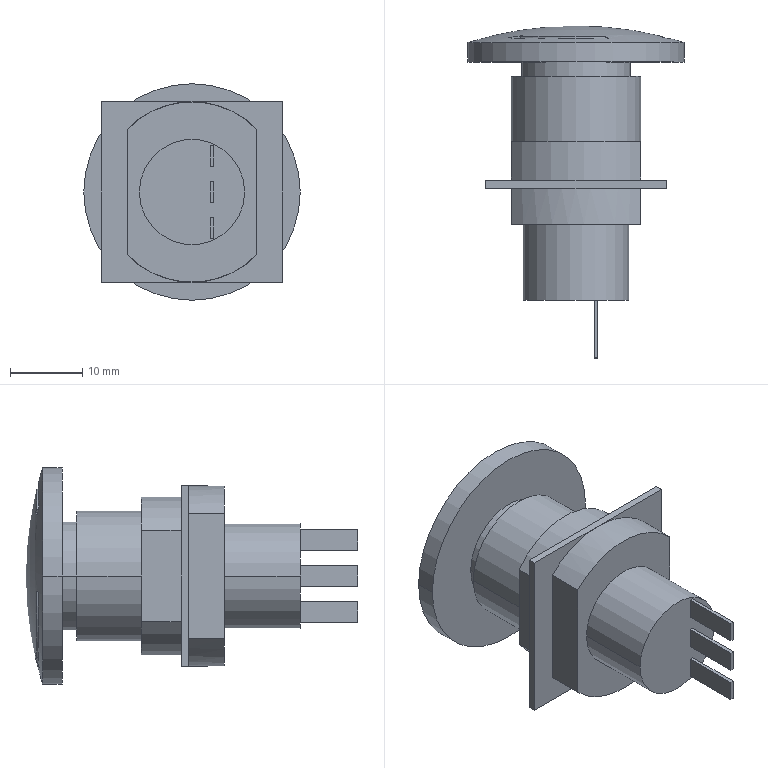Part | NX | 1 solid | 69 faces | box 30 x 46 x 30 mm | volume 11695 mm3 | plane 50 | cylinder 18 | sphere 1 | commonest cylinder face diameters 24 x3 26 x3 14.6 x2 15 x2 18 x2 22 x2